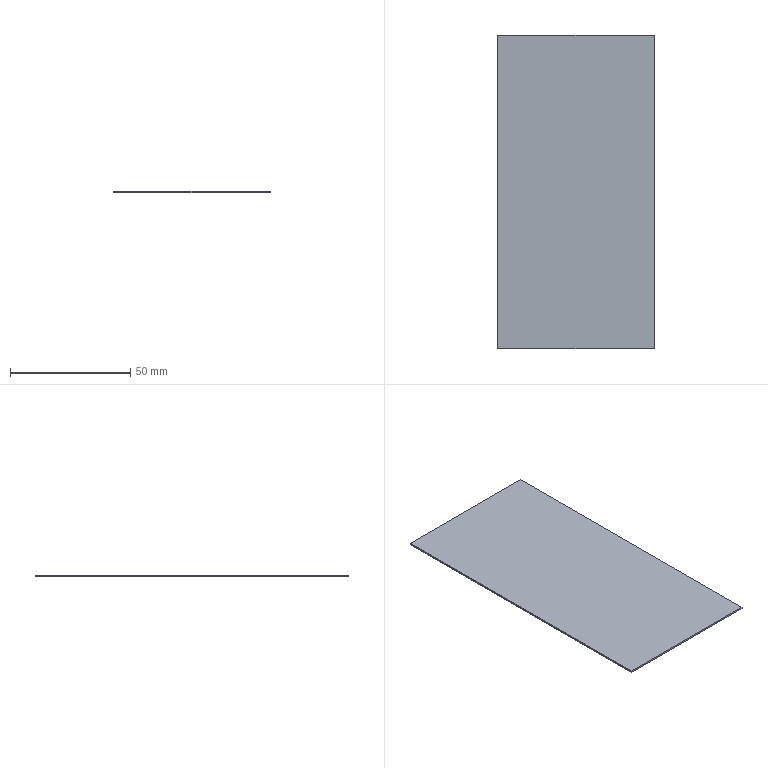Part | STEP file | 0217_Work-A | 1 solid | 6 faces | box 65 x 130 x 0.7 mm | volume 5915 mm3 | plane 6
STEP:
#1=CARTESIAN_POINT('',(0.,0.,0.));
#2=DIRECTION('',(0.,0.,1.));
#3=DIRECTION('',(1.,0.,0.));
#4=AXIS2_PLACEMENT_3D('',#1,#2,#3);
#5=CARTESIAN_POINT('',(-32.5,130.,0.));
#6=VERTEX_POINT('',#5);
#7=CARTESIAN_POINT('',(-32.5,0.,0.));
#8=VERTEX_POINT('',#7);
#9=CARTESIAN_POINT('',(-32.5,0.,0.));
#10=DIRECTION('',(0.,-1.,0.));
#11=VECTOR('',#10,1.);
#12=LINE('',#9,#11);
#13=CARTESIAN_POINT('',(-32.5,0.,0.7));
#14=DIRECTION('',(1.,0.,0.));
#15=DIRECTION('',(0.,0.,-1.));
#16=AXIS2_PLACEMENT_3D('',#13,#14,#15);
#17=PLANE('',#16);
#18=CARTESIAN_POINT('',(0.7,0.));
#19=DIRECTION('',(0.,-1.));
#20=VECTOR('',#19,1.);
#21=LINE('',#18,#20);
#22=(GEOMETRIC_REPRESENTATION_CONTEXT(2)PARAMETRIC_REPRESENTATION_CONTEXT()REPRESENTATION_CONTEXT('',''));
#23=DEFINITIONAL_REPRESENTATION('',(#21),#22);
#24=PCURVE('',#17,#23);
#25=CARTESIAN_POINT('',(-32.5,130.,0.));
#26=DIRECTION('',(0.,0.,-1.));
#27=DIRECTION('',(-1.,0.,0.));
#28=AXIS2_PLACEMENT_3D('',#25,#26,#27);
#29=PLANE('',#28);
#30=CARTESIAN_POINT('',(0.,-130.));
#31=DIRECTION('',(0.,-1.));
#32=VECTOR('',#31,1.);
#33=LINE('',#30,#32);
#34=(GEOMETRIC_REPRESENTATION_CONTEXT(2)PARAMETRIC_REPRESENTATION_CONTEXT()REPRESENTATION_CONTEXT('',''));
#35=DEFINITIONAL_REPRESENTATION('',(#33),#34);
#36=PCURVE('',#29,#35);
#37=SURFACE_CURVE('',#12,(#24,#36),.PCURVE_S1.);
#38=EDGE_CURVE('',#6,#8,#37,.T.);
#39=ORIENTED_EDGE('',*,*,#38,.T.);
#40=CARTESIAN_POINT('',(-32.5,0.,0.7));
#41=VERTEX_POINT('',#40);
#42=CARTESIAN_POINT('',(-32.5,0.,0.7));
#43=DIRECTION('',(0.,0.,-1.));
#44=VECTOR('',#43,1.);
#45=LINE('',#42,#44);
#46=CARTESIAN_POINT('',(0.,0.));
#47=DIRECTION('',(1.,0.));
#48=VECTOR('',#47,1.);
#49=LINE('',#46,#48);
#50=(GEOMETRIC_REPRESENTATION_CONTEXT(2)PARAMETRIC_REPRESENTATION_CONTEXT()REPRESENTATION_CONTEXT('',''));
#51=DEFINITIONAL_REPRESENTATION('',(#49),#50);
#52=PCURVE('',#17,#51);
#53=CARTESIAN_POINT('',(-32.5,0.,0.7));
#54=DIRECTION('',(0.,1.,0.));
#55=DIRECTION('',(0.,0.,1.));
#56=AXIS2_PLACEMENT_3D('',#53,#54,#55);
#57=PLANE('',#56);
#58=CARTESIAN_POINT('',(0.,0.));
#59=DIRECTION('',(-1.,0.));
#60=VECTOR('',#59,1.);
#61=LINE('',#58,#60);
#62=(GEOMETRIC_REPRESENTATION_CONTEXT(2)PARAMETRIC_REPRESENTATION_CONTEXT()REPRESENTATION_CONTEXT('',''));
#63=DEFINITIONAL_REPRESENTATION('',(#61),#62);
#64=PCURVE('',#57,#63);
#65=SURFACE_CURVE('',#45,(#52,#64),.PCURVE_S1.);
#66=EDGE_CURVE('',#41,#8,#65,.T.);
#67=ORIENTED_EDGE('',*,*,#66,.F.);
#68=CARTESIAN_POINT('',(-32.5,130.,0.7));
#69=VERTEX_POINT('',#68);
#70=CARTESIAN_POINT('',(-32.5,0.,0.7));
#71=DIRECTION('',(0.,-1.,0.));
#72=VECTOR('',#71,1.);
#73=LINE('',#70,#72);
#74=CARTESIAN_POINT('',(0.,0.));
#75=DIRECTION('',(0.,-1.));
#76=VECTOR('',#75,1.);
#77=LINE('',#74,#76);
#78=(GEOMETRIC_REPRESENTATION_CONTEXT(2)PARAMETRIC_REPRESENTATION_CONTEXT()REPRESENTATION_CONTEXT('',''));
#79=DEFINITIONAL_REPRESENTATION('',(#77),#78);
#80=PCURVE('',#17,#79);
#81=CARTESIAN_POINT('',(-32.5,130.,0.7));
#82=DIRECTION('',(0.,0.,-1.));
#83=DIRECTION('',(-1.,0.,0.));
#84=AXIS2_PLACEMENT_3D('',#81,#82,#83);
#85=PLANE('',#84);
#86=CARTESIAN_POINT('',(0.,-130.));
#87=DIRECTION('',(0.,-1.));
#88=VECTOR('',#87,1.);
#89=LINE('',#86,#88);
#90=(GEOMETRIC_REPRESENTATION_CONTEXT(2)PARAMETRIC_REPRESENTATION_CONTEXT()REPRESENTATION_CONTEXT('',''));
#91=DEFINITIONAL_REPRESENTATION('',(#89),#90);
#92=PCURVE('',#85,#91);
#93=SURFACE_CURVE('',#73,(#80,#92),.PCURVE_S1.);
#94=EDGE_CURVE('',#69,#41,#93,.T.);
#95=ORIENTED_EDGE('',*,*,#94,.F.);
#96=CARTESIAN_POINT('',(-32.5,130.,0.7));
#97=DIRECTION('',(0.,0.,-1.));
#98=VECTOR('',#97,1.);
#99=LINE('',#96,#98);
#100=CARTESIAN_POINT('',(0.,130.));
#101=DIRECTION('',(1.,0.));
#102=VECTOR('',#101,1.);
#103=LINE('',#100,#102);
#104=(GEOMETRIC_REPRESENTATION_CONTEXT(2)PARAMETRIC_REPRESENTATION_CONTEXT()REPRESENTATION_CONTEXT('',''));
#105=DEFINITIONAL_REPRESENTATION('',(#103),#104);
#106=PCURVE('',#17,#105);
#107=CARTESIAN_POINT('',(-32.5,130.,0.7));
#108=DIRECTION('',(0.,-1.,0.));
#109=DIRECTION('',(0.,0.,-1.));
#110=AXIS2_PLACEMENT_3D('',#107,#108,#109);
#111=PLANE('',#110);
#112=CARTESIAN_POINT('',(0.,0.));
#113=DIRECTION('',(1.,0.));
#114=VECTOR('',#113,1.);
#115=LINE('',#112,#114);
#116=(GEOMETRIC_REPRESENTATION_CONTEXT(2)PARAMETRIC_REPRESENTATION_CONTEXT()REPRESENTATION_CONTEXT('',''));
#117=DEFINITIONAL_REPRESENTATION('',(#115),#116);
#118=PCURVE('',#111,#117);
#119=SURFACE_CURVE('',#99,(#106,#118),.PCURVE_S1.);
#120=EDGE_CURVE('',#69,#6,#119,.T.);
#121=ORIENTED_EDGE('',*,*,#120,.T.);
#122=EDGE_LOOP('',(#39,#67,#95,#121));
#123=FACE_BOUND('',#122,.T.);
#124=ADVANCED_FACE('',(#123),#17,.F.);
#125=CARTESIAN_POINT('',(32.5,0.,0.));
#126=VERTEX_POINT('',#125);
#127=CARTESIAN_POINT('',(-32.5,0.,0.));
#128=DIRECTION('',(1.,0.,0.));
#129=VECTOR('',#128,1.);
#130=LINE('',#127,#129);
#131=CARTESIAN_POINT('',(-0.7,0.));
#132=DIRECTION('',(0.,1.));
#133=VECTOR('',#132,1.);
#134=LINE('',#131,#133);
#135=(GEOMETRIC_REPRESENTATION_CONTEXT(2)PARAMETRIC_REPRESENTATION_CONTEXT()REPRESENTATION_CONTEXT('',''));
#136=DEFINITIONAL_REPRESENTATION('',(#134),#135);
#137=PCURVE('',#57,#136);
#138=CARTESIAN_POINT('',(0.,-130.));
#139=DIRECTION('',(-1.,0.));
#140=VECTOR('',#139,1.);
#141=LINE('',#138,#140);
#142=(GEOMETRIC_REPRESENTATION_CONTEXT(2)PARAMETRIC_REPRESENTATION_CONTEXT()REPRESENTATION_CONTEXT('',''));
#143=DEFINITIONAL_REPRESENTATION('',(#141),#142);
#144=PCURVE('',#29,#143);
#145=SURFACE_CURVE('',#130,(#137,#144),.PCURVE_S1.);
#146=EDGE_CURVE('',#8,#126,#145,.T.);
#147=ORIENTED_EDGE('',*,*,#146,.T.);
#148=CARTESIAN_POINT('',(32.5,0.,0.7));
#149=VERTEX_POINT('',#148);
#150=CARTESIAN_POINT('',(32.5,0.,0.7));
#151=DIRECTION('',(0.,0.,-1.));
#152=VECTOR('',#151,1.);
#153=LINE('',#150,#152);
#154=CARTESIAN_POINT('',(0.,65.));
#155=DIRECTION('',(-1.,0.));
#156=VECTOR('',#155,1.);
#157=LINE('',#154,#156);
#158=(GEOMETRIC_REPRESENTATION_CONTEXT(2)PARAMETRIC_REPRESENTATION_CONTEXT()REPRESENTATION_CONTEXT('',''));
#159=DEFINITIONAL_REPRESENTATION('',(#157),#158);
#160=PCURVE('',#57,#159);
#161=CARTESIAN_POINT('',(32.5,0.,0.7));
#162=DIRECTION('',(-1.,0.,0.));
#163=DIRECTION('',(0.,0.,1.));
#164=AXIS2_PLACEMENT_3D('',#161,#162,#163);
#165=PLANE('',#164);
#166=CARTESIAN_POINT('',(0.,0.));
#167=DIRECTION('',(-1.,0.));
#168=VECTOR('',#167,1.);
#169=LINE('',#166,#168);
#170=(GEOMETRIC_REPRESENTATION_CONTEXT(2)PARAMETRIC_REPRESENTATION_CONTEXT()REPRESENTATION_CONTEXT('',''));
#171=DEFINITIONAL_REPRESENTATION('',(#169),#170);
#172=PCURVE('',#165,#171);
#173=SURFACE_CURVE('',#153,(#160,#172),.PCURVE_S1.);
#174=EDGE_CURVE('',#149,#126,#173,.T.);
#175=ORIENTED_EDGE('',*,*,#174,.F.);
#176=CARTESIAN_POINT('',(-32.5,0.,0.7));
#177=DIRECTION('',(1.,0.,0.));
#178=VECTOR('',#177,1.);
#179=LINE('',#176,#178);
#180=CARTESIAN_POINT('',(0.,0.));
#181=DIRECTION('',(0.,1.));
#182=VECTOR('',#181,1.);
#183=LINE('',#180,#182);
#184=(GEOMETRIC_REPRESENTATION_CONTEXT(2)PARAMETRIC_REPRESENTATION_CONTEXT()REPRESENTATION_CONTEXT('',''));
#185=DEFINITIONAL_REPRESENTATION('',(#183),#184);
#186=PCURVE('',#57,#185);
#187=CARTESIAN_POINT('',(0.,-130.));
#188=DIRECTION('',(-1.,0.));
#189=VECTOR('',#188,1.);
#190=LINE('',#187,#189);
#191=(GEOMETRIC_REPRESENTATION_CONTEXT(2)PARAMETRIC_REPRESENTATION_CONTEXT()REPRESENTATION_CONTEXT('',''));
#192=DEFINITIONAL_REPRESENTATION('',(#190),#191);
#193=PCURVE('',#85,#192);
#194=SURFACE_CURVE('',#179,(#186,#193),.PCURVE_S1.);
#195=EDGE_CURVE('',#41,#149,#194,.T.);
#196=ORIENTED_EDGE('',*,*,#195,.F.);
#197=ORIENTED_EDGE('',*,*,#66,.T.);
#198=EDGE_LOOP('',(#147,#175,#196,#197));
#199=FACE_BOUND('',#198,.T.);
#200=ADVANCED_FACE('',(#199),#57,.F.);
#201=CARTESIAN_POINT('',(32.5,130.,0.));
#202=VERTEX_POINT('',#201);
#203=CARTESIAN_POINT('',(32.5,0.,0.));
#204=DIRECTION('',(0.,1.,0.));
#205=VECTOR('',#204,1.);
#206=LINE('',#203,#205);
#207=CARTESIAN_POINT('',(-0.7,0.));
#208=DIRECTION('',(0.,1.));
#209=VECTOR('',#208,1.);
#210=LINE('',#207,#209);
#211=(GEOMETRIC_REPRESENTATION_CONTEXT(2)PARAMETRIC_REPRESENTATION_CONTEXT()REPRESENTATION_CONTEXT('',''));
#212=DEFINITIONAL_REPRESENTATION('',(#210),#211);
#213=PCURVE('',#165,#212);
#214=CARTESIAN_POINT('',(-65.,-130.));
#215=DIRECTION('',(0.,1.));
#216=VECTOR('',#215,1.);
#217=LINE('',#214,#216);
#218=(GEOMETRIC_REPRESENTATION_CONTEXT(2)PARAMETRIC_REPRESENTATION_CONTEXT()REPRESENTATION_CONTEXT('',''));
#219=DEFINITIONAL_REPRESENTATION('',(#217),#218);
#220=PCURVE('',#29,#219);
#221=SURFACE_CURVE('',#206,(#213,#220),.PCURVE_S1.);
#222=EDGE_CURVE('',#126,#202,#221,.T.);
#223=ORIENTED_EDGE('',*,*,#222,.T.);
#224=CARTESIAN_POINT('',(32.5,130.,0.7));
#225=VERTEX_POINT('',#224);
#226=CARTESIAN_POINT('',(32.5,130.,0.7));
#227=DIRECTION('',(0.,0.,-1.));
#228=VECTOR('',#227,1.);
#229=LINE('',#226,#228);
#230=CARTESIAN_POINT('',(0.,130.));
#231=DIRECTION('',(-1.,0.));
#232=VECTOR('',#231,1.);
#233=LINE('',#230,#232);
#234=(GEOMETRIC_REPRESENTATION_CONTEXT(2)PARAMETRIC_REPRESENTATION_CONTEXT()REPRESENTATION_CONTEXT('',''));
#235=DEFINITIONAL_REPRESENTATION('',(#233),#234);
#236=PCURVE('',#165,#235);
#237=CARTESIAN_POINT('',(0.,65.));
#238=DIRECTION('',(1.,0.));
#239=VECTOR('',#238,1.);
#240=LINE('',#237,#239);
#241=(GEOMETRIC_REPRESENTATION_CONTEXT(2)PARAMETRIC_REPRESENTATION_CONTEXT()REPRESENTATION_CONTEXT('',''));
#242=DEFINITIONAL_REPRESENTATION('',(#240),#241);
#243=PCURVE('',#111,#242);
#244=SURFACE_CURVE('',#229,(#236,#243),.PCURVE_S1.);
#245=EDGE_CURVE('',#225,#202,#244,.T.);
#246=ORIENTED_EDGE('',*,*,#245,.F.);
#247=CARTESIAN_POINT('',(32.5,0.,0.7));
#248=DIRECTION('',(0.,1.,0.));
#249=VECTOR('',#248,1.);
#250=LINE('',#247,#249);
#251=CARTESIAN_POINT('',(0.,0.));
#252=DIRECTION('',(0.,1.));
#253=VECTOR('',#252,1.);
#254=LINE('',#251,#253);
#255=(GEOMETRIC_REPRESENTATION_CONTEXT(2)PARAMETRIC_REPRESENTATION_CONTEXT()REPRESENTATION_CONTEXT('',''));
#256=DEFINITIONAL_REPRESENTATION('',(#254),#255);
#257=PCURVE('',#165,#256);
#258=CARTESIAN_POINT('',(-65.,-130.));
#259=DIRECTION('',(0.,1.));
#260=VECTOR('',#259,1.);
#261=LINE('',#258,#260);
#262=(GEOMETRIC_REPRESENTATION_CONTEXT(2)PARAMETRIC_REPRESENTATION_CONTEXT()REPRESENTATION_CONTEXT('',''));
#263=DEFINITIONAL_REPRESENTATION('',(#261),#262);
#264=PCURVE('',#85,#263);
#265=SURFACE_CURVE('',#250,(#257,#264),.PCURVE_S1.);
#266=EDGE_CURVE('',#149,#225,#265,.T.);
#267=ORIENTED_EDGE('',*,*,#266,.F.);
#268=ORIENTED_EDGE('',*,*,#174,.T.);
#269=EDGE_LOOP('',(#223,#246,#267,#268));
#270=FACE_BOUND('',#269,.T.);
#271=ADVANCED_FACE('',(#270),#165,.F.);
#272=CARTESIAN_POINT('',(-32.5,130.,0.));
#273=DIRECTION('',(-1.,0.,0.));
#274=VECTOR('',#273,1.);
#275=LINE('',#272,#274);
#276=CARTESIAN_POINT('',(0.7,0.));
#277=DIRECTION('',(0.,-1.));
#278=VECTOR('',#277,1.);
#279=LINE('',#276,#278);
#280=(GEOMETRIC_REPRESENTATION_CONTEXT(2)PARAMETRIC_REPRESENTATION_CONTEXT()REPRESENTATION_CONTEXT('',''));
#281=DEFINITIONAL_REPRESENTATION('',(#279),#280);
#282=PCURVE('',#111,#281);
#283=CARTESIAN_POINT('',(0.,0.));
#284=DIRECTION('',(1.,0.));
#285=VECTOR('',#284,1.);
#286=LINE('',#283,#285);
#287=(GEOMETRIC_REPRESENTATION_CONTEXT(2)PARAMETRIC_REPRESENTATION_CONTEXT()REPRESENTATION_CONTEXT('',''));
#288=DEFINITIONAL_REPRESENTATION('',(#286),#287);
#289=PCURVE('',#29,#288);
#290=SURFACE_CURVE('',#275,(#282,#289),.PCURVE_S1.);
#291=EDGE_CURVE('',#202,#6,#290,.T.);
#292=ORIENTED_EDGE('',*,*,#291,.T.);
#293=ORIENTED_EDGE('',*,*,#120,.F.);
#294=CARTESIAN_POINT('',(-32.5,130.,0.7));
#295=DIRECTION('',(-1.,0.,0.));
#296=VECTOR('',#295,1.);
#297=LINE('',#294,#296);
#298=CARTESIAN_POINT('',(0.,0.));
#299=DIRECTION('',(0.,-1.));
#300=VECTOR('',#299,1.);
#301=LINE('',#298,#300);
#302=(GEOMETRIC_REPRESENTATION_CONTEXT(2)PARAMETRIC_REPRESENTATION_CONTEXT()REPRESENTATION_CONTEXT('',''));
#303=DEFINITIONAL_REPRESENTATION('',(#301),#302);
#304=PCURVE('',#111,#303);
#305=CARTESIAN_POINT('',(0.,0.));
#306=DIRECTION('',(1.,0.));
#307=VECTOR('',#306,1.);
#308=LINE('',#305,#307);
#309=(GEOMETRIC_REPRESENTATION_CONTEXT(2)PARAMETRIC_REPRESENTATION_CONTEXT()REPRESENTATION_CONTEXT('',''));
#310=DEFINITIONAL_REPRESENTATION('',(#308),#309);
#311=PCURVE('',#85,#310);
#312=SURFACE_CURVE('',#297,(#304,#311),.PCURVE_S1.);
#313=EDGE_CURVE('',#225,#69,#312,.T.);
#314=ORIENTED_EDGE('',*,*,#313,.F.);
#315=ORIENTED_EDGE('',*,*,#245,.T.);
#316=EDGE_LOOP('',(#292,#293,#314,#315));
#317=FACE_BOUND('',#316,.T.);
#318=ADVANCED_FACE('',(#317),#111,.F.);
#319=ORIENTED_EDGE('',*,*,#94,.T.);
#320=ORIENTED_EDGE('',*,*,#195,.T.);
#321=ORIENTED_EDGE('',*,*,#266,.T.);
#322=ORIENTED_EDGE('',*,*,#313,.T.);
#323=EDGE_LOOP('',(#319,#320,#321,#322));
#324=FACE_BOUND('',#323,.T.);
#325=ADVANCED_FACE('',(#324),#85,.F.);
#326=ORIENTED_EDGE('',*,*,#38,.F.);
#327=ORIENTED_EDGE('',*,*,#291,.F.);
#328=ORIENTED_EDGE('',*,*,#222,.F.);
#329=ORIENTED_EDGE('',*,*,#146,.F.);
#330=EDGE_LOOP('',(#326,#327,#328,#329));
#331=FACE_BOUND('',#330,.T.);
#332=ADVANCED_FACE('',(#331),#29,.T.);
#333=CLOSED_SHELL('',(#124,#200,#271,#318,#325,#332));
#334=MANIFOLD_SOLID_BREP('',#333);
#335=(LENGTH_UNIT()NAMED_UNIT(*)SI_UNIT(.MILLI.,.METRE.));
#336=UNCERTAINTY_MEASURE_WITH_UNIT(LENGTH_MEASURE(0.0000001),#335,'','');
#337=(NAMED_UNIT(*)PLANE_ANGLE_UNIT()SI_UNIT($,.RADIAN.));
#338=(NAMED_UNIT(*)SI_UNIT($,.STERADIAN.)SOLID_ANGLE_UNIT());
#339=(GEOMETRIC_REPRESENTATION_CONTEXT(3)GLOBAL_UNCERTAINTY_ASSIGNED_CONTEXT((#336))GLOBAL_UNIT_ASSIGNED_CONTEXT((#335,#337,#338))REPRESENTATION_CONTEXT('',''));
#340=ADVANCED_BREP_SHAPE_REPRESENTATION('',(#4,#334),#339);